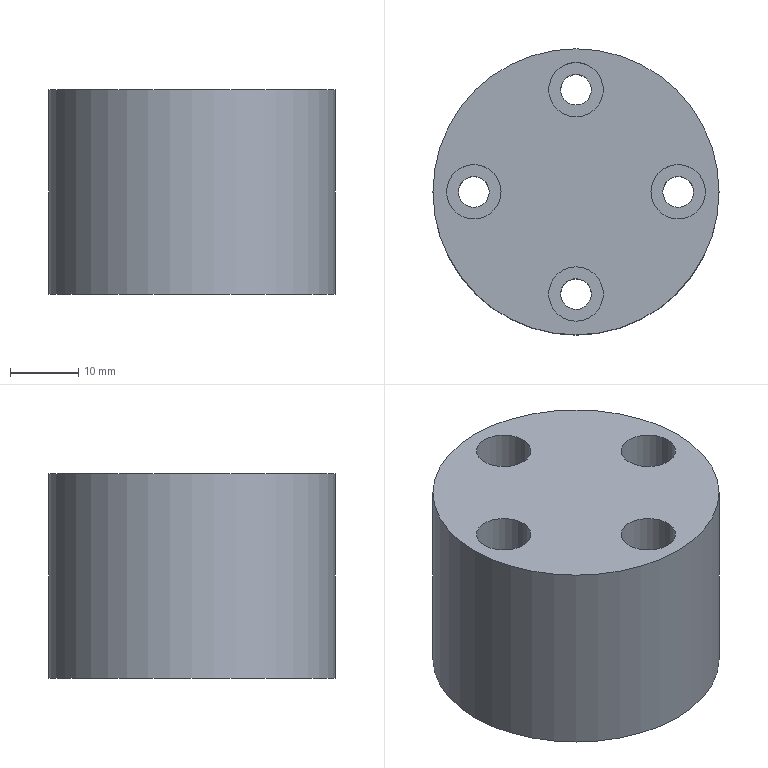CAM job | NX | 3-axis milling, drilling | part box 42 x 42 x 30 mm | stock box 42 x 42 x 30 mm
Tools:
number,name,description,diameter,corner_radius,flute_length,length,flutes
1,ZXZ,Milling Tool-5 Parameters,6.0,0.0,50.0,75.0,2
7,D6A45,Milling Tool-5 Parameters,6.0,0.0,3.0,3.0,2
2,4.5ZT,Drilling Tool,4.5,0.0,35.0,50.0,2
6,D6,Milling Tool-5 Parameters,6.0,0.0,50.0,75.0,2
Operations:
program,operation,operation_type,tool,method,geometry_group,spindle_rpm,surface_speed,feed_per_tooth,feed_cut,feed_plunge,cut_length_mm,path_length_mm,cut_time_min,machine_time_min
1,DRILLING,Operation,ZXZ,METHOD,A,3000.0,56.0,0.0333,200.0,0.0,16.0,165.273,0.08,0.0949
1,DRILLING_COPY,Operation,4.5ZT,METHOD,A,2000.0,28.0,0.03,120.0,0.0,143.408,420.088,1.195,1.223
1,HOLE_MILLING,CylinderMilling,D6,METHOD,A,4500.0,84.0,0.1556,1400.0,100.0,1671.534,1997.174,1.194,1.226
1,ZLEVEL_PROFILE_1_COPY_1,ZLevelMilling,D6A45,METHOD,A,7500.0,141.0,0.0667,1000.0,100.0,105.156,435.622,0.1052,0.1382